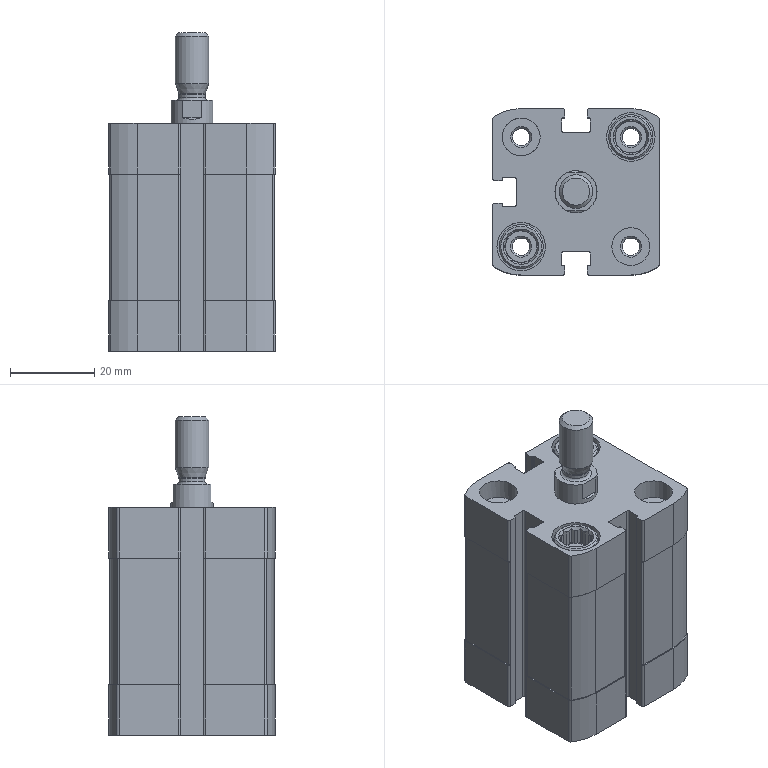Part | NX | features BREP 2 | 2 solids | 350 faces | box 39.5 x 39.5 x 75.5 mm | volume 65576 mm3 | plane 231 | cylinder 97 | cone 20 | torus 2 | commonest cylinder face diameters 0.8 x24 0.4 x12 1.6 x12 23.4 x12 4.134 x10 9 x5